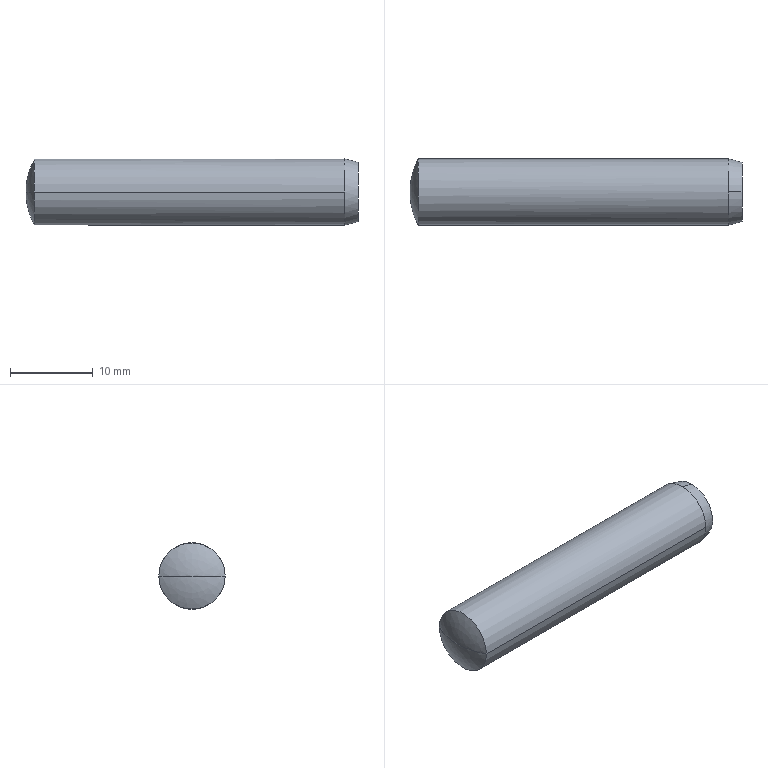Part | STEP file | DIN EN 22338 A - withdrawn 8 m6 x 40 - A | 1 solid | 7 faces | box 40 x 8 x 8 mm | volume 1978 mm3 | spline 2 | cylinder 2 | cone 2 | plane 1 | commonest cylinder face diameters 8 x2
STEP:
#1=CARTESIAN_POINT('',(0.,0.,0.));
#2=DIRECTION('',(0.,0.,1.));
#3=DIRECTION('',(1.,0.,0.));
#4=AXIS2_PLACEMENT_3D('',#1,#2,#3);
#5=CARTESIAN_POINT('',(1.,-4.,0.));
#6=VERTEX_POINT('',#5);
#7=CARTESIAN_POINT('',(1.,4.,0.));
#8=VERTEX_POINT('',#7);
#9=CARTESIAN_POINT('',(1.,0.,0.));
#10=DIRECTION('',(1.,0.,0.));
#11=DIRECTION('',(0.,1.,0.));
#12=AXIS2_PLACEMENT_3D('',#9,#10,#11);
#13=CIRCLE('',#12,4.);
#14=CARTESIAN_POINT('',(1.,-4.,0.));
#15=CARTESIAN_POINT('',(1.,-4.,-8.));
#16=CARTESIAN_POINT('',(1.,4.,-8.));
#17=CARTESIAN_POINT('',(1.,4.,0.));
#18=CARTESIAN_POINT('',(0.3401,-2.763,0.));
#19=CARTESIAN_POINT('',(0.3401,-2.763,-5.525));
#20=CARTESIAN_POINT('',(0.3401,2.763,-5.525));
#21=CARTESIAN_POINT('',(0.3401,2.763,0.));
#22=CARTESIAN_POINT('',(0.,-1.402,0.));
#23=CARTESIAN_POINT('',(0.,-1.402,-2.805));
#24=CARTESIAN_POINT('',(0.,1.402,-2.805));
#25=CARTESIAN_POINT('',(0.,1.402,0.));
#26=CARTESIAN_POINT('',(0.,0.,0.));
#27=CARTESIAN_POINT('',(0.,0.,0.));
#28=CARTESIAN_POINT('',(0.,0.,0.));
#29=CARTESIAN_POINT('',(0.,0.,0.));
#30=(BOUNDED_SURFACE()B_SPLINE_SURFACE(3,3,((#14,#15,#16,#17),(#18,#19,#20,#21),(#22,#23,#24,#25),(#26,#27,#28,#29)),.UNSPECIFIED.,.F.,.F.,.F.)B_SPLINE_SURFACE_WITH_KNOTS((4,4),(4,4),(0.,1.),(0.,1.),.PIECEWISE_BEZIER_KNOTS.)GEOMETRIC_REPRESENTATION_ITEM()RATIONAL_B_SPLINE_SURFACE(((1.,0.3333,0.3333,1.),(0.9801,0.3267,0.3267,0.9801),(0.9801,0.3267,0.3267,0.9801),(1.,0.3333,0.3333,1.)))REPRESENTATION_ITEM('')SURFACE());
#31=CARTESIAN_POINT('',(0.,0.));
#32=CARTESIAN_POINT('',(0.,0.02375));
#33=CARTESIAN_POINT('',(0.,0.06805));
#34=CARTESIAN_POINT('',(0.,0.1267));
#35=CARTESIAN_POINT('',(0.,0.1794));
#36=CARTESIAN_POINT('',(0.,0.2276));
#37=CARTESIAN_POINT('',(0.,0.2721));
#38=CARTESIAN_POINT('',(0.,0.3139));
#39=CARTESIAN_POINT('',(0.,0.3535));
#40=CARTESIAN_POINT('',(0.,0.3914));
#41=CARTESIAN_POINT('',(0.,0.4282));
#42=CARTESIAN_POINT('',(0.,0.4643));
#43=CARTESIAN_POINT('',(0.,0.5));
#44=CARTESIAN_POINT('',(0.,0.5357));
#45=CARTESIAN_POINT('',(0.,0.5718));
#46=CARTESIAN_POINT('',(0.,0.6086));
#47=CARTESIAN_POINT('',(0.,0.6465));
#48=CARTESIAN_POINT('',(0.,0.6861));
#49=CARTESIAN_POINT('',(0.,0.7279));
#50=CARTESIAN_POINT('',(0.,0.7724));
#51=CARTESIAN_POINT('',(0.,0.8206));
#52=CARTESIAN_POINT('',(0.,0.8733));
#53=CARTESIAN_POINT('',(0.,0.9319));
#54=CARTESIAN_POINT('',(0.,0.9763));
#55=CARTESIAN_POINT('',(0.,1.));
#56=B_SPLINE_CURVE_WITH_KNOTS('',3,(#31,#32,#33,#34,#35,#36,#37,#38,#39,#40,#41,#42,#43,#44,#45,#46,#47,#48,#49,#50,#51,#52,#53,#54,#55),.UNSPECIFIED.,.F.,.F.,(4,1,1,1,1,1,1,1,1,1,1,1,1,1,1,1,1,1,1,1,1,1,4),(3.142,3.284,3.427,3.57,3.713,3.856,3.998,4.141,4.284,4.427,4.57,4.712,4.855,4.998,5.141,5.284,5.426,5.569,5.712,5.855,5.998,6.14,6.283),.QUASI_UNIFORM_KNOTS.);
#57=(GEOMETRIC_REPRESENTATION_CONTEXT(2)PARAMETRIC_REPRESENTATION_CONTEXT()REPRESENTATION_CONTEXT('',''));
#58=DEFINITIONAL_REPRESENTATION('',(#56),#57);
#59=PCURVE('',#30,#58);
#60=CARTESIAN_POINT('',(19.7,0.,0.));
#61=DIRECTION('',(1.,0.,0.));
#62=DIRECTION('',(0.,1.,0.));
#63=AXIS2_PLACEMENT_3D('',#60,#61,#62);
#64=CYLINDRICAL_SURFACE('',#63,4.);
#65=CARTESIAN_POINT('',(0.,-18.7));
#66=DIRECTION('',(1.,0.));
#67=VECTOR('',#66,1.);
#68=LINE('',#65,#67);
#69=(GEOMETRIC_REPRESENTATION_CONTEXT(2)PARAMETRIC_REPRESENTATION_CONTEXT()REPRESENTATION_CONTEXT('',''));
#70=DEFINITIONAL_REPRESENTATION('',(#68),#69);
#71=PCURVE('',#64,#70);
#72=SURFACE_CURVE('',#13,(#59,#71),.PCURVE_S1.);
#73=EDGE_CURVE('',#6,#8,#72,.T.);
#74=ORIENTED_EDGE('',*,*,#73,.F.);
#75=CARTESIAN_POINT('',(0.,0.,0.));
#76=VERTEX_POINT('',#75);
#77=CARTESIAN_POINT('',(8.5,0.,0.));
#78=DIRECTION('',(0.,0.,-1.));
#79=DIRECTION('',(1.,0.,0.));
#80=AXIS2_PLACEMENT_3D('',#77,#78,#79);
#81=CIRCLE('',#80,8.5);
#82=CARTESIAN_POINT('',(0.,0.));
#83=CARTESIAN_POINT('',(0.0153,0.));
#84=CARTESIAN_POINT('',(0.04587,0.));
#85=CARTESIAN_POINT('',(0.09161,0.));
#86=CARTESIAN_POINT('',(0.1372,0.));
#87=CARTESIAN_POINT('',(0.1828,0.));
#88=CARTESIAN_POINT('',(0.2282,0.));
#89=CARTESIAN_POINT('',(0.2736,0.));
#90=CARTESIAN_POINT('',(0.319,0.));
#91=CARTESIAN_POINT('',(0.3643,0.));
#92=CARTESIAN_POINT('',(0.4095,0.));
#93=CARTESIAN_POINT('',(0.4548,0.));
#94=CARTESIAN_POINT('',(0.5,0.));
#95=CARTESIAN_POINT('',(0.5452,0.));
#96=CARTESIAN_POINT('',(0.5905,0.));
#97=CARTESIAN_POINT('',(0.6357,0.));
#98=CARTESIAN_POINT('',(0.681,0.));
#99=CARTESIAN_POINT('',(0.7264,0.));
#100=CARTESIAN_POINT('',(0.7718,0.));
#101=CARTESIAN_POINT('',(0.8172,0.));
#102=CARTESIAN_POINT('',(0.8628,0.));
#103=CARTESIAN_POINT('',(0.9084,0.));
#104=CARTESIAN_POINT('',(0.9541,0.));
#105=CARTESIAN_POINT('',(0.9847,0.));
#106=CARTESIAN_POINT('',(1.,0.));
#107=B_SPLINE_CURVE_WITH_KNOTS('',3,(#82,#83,#84,#85,#86,#87,#88,#89,#90,#91,#92,#93,#94,#95,#96,#97,#98,#99,#100,#101,#102,#103,#104,#105,#106),.UNSPECIFIED.,.F.,.F.,(4,1,1,1,1,1,1,1,1,1,1,1,1,1,1,1,1,1,1,1,1,1,4),(2.652,2.674,2.696,2.718,2.741,2.763,2.785,2.808,2.83,2.852,2.874,2.897,2.919,2.941,2.963,2.986,3.008,3.03,3.053,3.075,3.097,3.119,3.142),.QUASI_UNIFORM_KNOTS.);
#108=(GEOMETRIC_REPRESENTATION_CONTEXT(2)PARAMETRIC_REPRESENTATION_CONTEXT()REPRESENTATION_CONTEXT('',''));
#109=DEFINITIONAL_REPRESENTATION('',(#107),#108);
#110=PCURVE('',#30,#109);
#111=CARTESIAN_POINT('',(1.,4.,0.));
#112=CARTESIAN_POINT('',(1.,4.,8.));
#113=CARTESIAN_POINT('',(1.,-4.,8.));
#114=CARTESIAN_POINT('',(1.,-4.,0.));
#115=CARTESIAN_POINT('',(0.3401,2.763,0.));
#116=CARTESIAN_POINT('',(0.3401,2.763,5.525));
#117=CARTESIAN_POINT('',(0.3401,-2.763,5.525));
#118=CARTESIAN_POINT('',(0.3401,-2.763,0.));
#119=CARTESIAN_POINT('',(0.,1.402,0.));
#120=CARTESIAN_POINT('',(0.,1.402,2.805));
#121=CARTESIAN_POINT('',(0.,-1.402,2.805));
#122=CARTESIAN_POINT('',(0.,-1.402,0.));
#123=CARTESIAN_POINT('',(0.,0.,0.));
#124=CARTESIAN_POINT('',(0.,0.,0.));
#125=CARTESIAN_POINT('',(0.,0.,0.));
#126=CARTESIAN_POINT('',(0.,0.,0.));
#127=(BOUNDED_SURFACE()B_SPLINE_SURFACE(3,3,((#111,#112,#113,#114),(#115,#116,#117,#118),(#119,#120,#121,#122),(#123,#124,#125,#126)),.UNSPECIFIED.,.F.,.F.,.F.)B_SPLINE_SURFACE_WITH_KNOTS((4,4),(4,4),(0.,1.),(0.,1.),.PIECEWISE_BEZIER_KNOTS.)GEOMETRIC_REPRESENTATION_ITEM()RATIONAL_B_SPLINE_SURFACE(((1.,0.3333,0.3333,1.),(0.9801,0.3267,0.3267,0.9801),(0.9801,0.3267,0.3267,0.9801),(1.,0.3333,0.3333,1.)))REPRESENTATION_ITEM('')SURFACE());
#128=CARTESIAN_POINT('',(0.,1.));
#129=CARTESIAN_POINT('',(0.0153,1.));
#130=CARTESIAN_POINT('',(0.04587,1.));
#131=CARTESIAN_POINT('',(0.09161,1.));
#132=CARTESIAN_POINT('',(0.1372,1.));
#133=CARTESIAN_POINT('',(0.1828,1.));
#134=CARTESIAN_POINT('',(0.2282,1.));
#135=CARTESIAN_POINT('',(0.2736,1.));
#136=CARTESIAN_POINT('',(0.319,1.));
#137=CARTESIAN_POINT('',(0.3643,1.));
#138=CARTESIAN_POINT('',(0.4095,1.));
#139=CARTESIAN_POINT('',(0.4548,1.));
#140=CARTESIAN_POINT('',(0.5,1.));
#141=CARTESIAN_POINT('',(0.5452,1.));
#142=CARTESIAN_POINT('',(0.5905,1.));
#143=CARTESIAN_POINT('',(0.6357,1.));
#144=CARTESIAN_POINT('',(0.681,1.));
#145=CARTESIAN_POINT('',(0.7264,1.));
#146=CARTESIAN_POINT('',(0.7718,1.));
#147=CARTESIAN_POINT('',(0.8172,1.));
#148=CARTESIAN_POINT('',(0.8628,1.));
#149=CARTESIAN_POINT('',(0.9084,1.));
#150=CARTESIAN_POINT('',(0.9541,1.));
#151=CARTESIAN_POINT('',(0.9847,1.));
#152=CARTESIAN_POINT('',(1.,1.));
#153=B_SPLINE_CURVE_WITH_KNOTS('',3,(#128,#129,#130,#131,#132,#133,#134,#135,#136,#137,#138,#139,#140,#141,#142,#143,#144,#145,#146,#147,#148,#149,#150,#151,#152),.UNSPECIFIED.,.F.,.F.,(4,1,1,1,1,1,1,1,1,1,1,1,1,1,1,1,1,1,1,1,1,1,4),(2.652,2.674,2.696,2.718,2.741,2.763,2.785,2.808,2.83,2.852,2.874,2.897,2.919,2.941,2.963,2.986,3.008,3.03,3.053,3.075,3.097,3.119,3.142),.QUASI_UNIFORM_KNOTS.);
#154=(GEOMETRIC_REPRESENTATION_CONTEXT(2)PARAMETRIC_REPRESENTATION_CONTEXT()REPRESENTATION_CONTEXT('',''));
#155=DEFINITIONAL_REPRESENTATION('',(#153),#154);
#156=PCURVE('',#127,#155);
#157=SURFACE_CURVE('',#81,(#110,#156),.PCURVE_S1.);
#158=EDGE_CURVE('',#6,#76,#157,.T.);
#159=ORIENTED_EDGE('',*,*,#158,.T.);
#160=CARTESIAN_POINT('',(8.5,0.,0.));
#161=DIRECTION('',(0.,0.,1.));
#162=DIRECTION('',(1.,0.,0.));
#163=AXIS2_PLACEMENT_3D('',#160,#161,#162);
#164=CIRCLE('',#163,8.5);
#165=CARTESIAN_POINT('',(0.,1.));
#166=CARTESIAN_POINT('',(0.0153,1.));
#167=CARTESIAN_POINT('',(0.04587,1.));
#168=CARTESIAN_POINT('',(0.09161,1.));
#169=CARTESIAN_POINT('',(0.1372,1.));
#170=CARTESIAN_POINT('',(0.1828,1.));
#171=CARTESIAN_POINT('',(0.2282,1.));
#172=CARTESIAN_POINT('',(0.2736,1.));
#173=CARTESIAN_POINT('',(0.319,1.));
#174=CARTESIAN_POINT('',(0.3643,1.));
#175=CARTESIAN_POINT('',(0.4095,1.));
#176=CARTESIAN_POINT('',(0.4548,1.));
#177=CARTESIAN_POINT('',(0.5,1.));
#178=CARTESIAN_POINT('',(0.5452,1.));
#179=CARTESIAN_POINT('',(0.5905,1.));
#180=CARTESIAN_POINT('',(0.6357,1.));
#181=CARTESIAN_POINT('',(0.681,1.));
#182=CARTESIAN_POINT('',(0.7264,1.));
#183=CARTESIAN_POINT('',(0.7718,1.));
#184=CARTESIAN_POINT('',(0.8172,1.));
#185=CARTESIAN_POINT('',(0.8628,1.));
#186=CARTESIAN_POINT('',(0.9084,1.));
#187=CARTESIAN_POINT('',(0.9541,1.));
#188=CARTESIAN_POINT('',(0.9847,1.));
#189=CARTESIAN_POINT('',(1.,1.));
#190=B_SPLINE_CURVE_WITH_KNOTS('',3,(#165,#166,#167,#168,#169,#170,#171,#172,#173,#174,#175,#176,#177,#178,#179,#180,#181,#182,#183,#184,#185,#186,#187,#188,#189),.UNSPECIFIED.,.F.,.F.,(4,1,1,1,1,1,1,1,1,1,1,1,1,1,1,1,1,1,1,1,1,1,4),(2.652,2.674,2.696,2.718,2.741,2.763,2.785,2.808,2.83,2.852,2.874,2.897,2.919,2.941,2.963,2.986,3.008,3.03,3.053,3.075,3.097,3.119,3.142),.QUASI_UNIFORM_KNOTS.);
#191=(GEOMETRIC_REPRESENTATION_CONTEXT(2)PARAMETRIC_REPRESENTATION_CONTEXT()REPRESENTATION_CONTEXT('',''));
#192=DEFINITIONAL_REPRESENTATION('',(#190),#191);
#193=PCURVE('',#30,#192);
#194=CARTESIAN_POINT('',(0.,0.));
#195=CARTESIAN_POINT('',(0.0153,0.));
#196=CARTESIAN_POINT('',(0.04587,0.));
#197=CARTESIAN_POINT('',(0.09161,0.));
#198=CARTESIAN_POINT('',(0.1372,0.));
#199=CARTESIAN_POINT('',(0.1828,0.));
#200=CARTESIAN_POINT('',(0.2282,0.));
#201=CARTESIAN_POINT('',(0.2736,0.));
#202=CARTESIAN_POINT('',(0.319,0.));
#203=CARTESIAN_POINT('',(0.3643,0.));
#204=CARTESIAN_POINT('',(0.4095,0.));
#205=CARTESIAN_POINT('',(0.4548,0.));
#206=CARTESIAN_POINT('',(0.5,0.));
#207=CARTESIAN_POINT('',(0.5452,0.));
#208=CARTESIAN_POINT('',(0.5905,0.));
#209=CARTESIAN_POINT('',(0.6357,0.));
#210=CARTESIAN_POINT('',(0.681,0.));
#211=CARTESIAN_POINT('',(0.7264,0.));
#212=CARTESIAN_POINT('',(0.7718,0.));
#213=CARTESIAN_POINT('',(0.8172,0.));
#214=CARTESIAN_POINT('',(0.8628,0.));
#215=CARTESIAN_POINT('',(0.9084,0.));
#216=CARTESIAN_POINT('',(0.9541,0.));
#217=CARTESIAN_POINT('',(0.9847,0.));
#218=CARTESIAN_POINT('',(1.,0.));
#219=B_SPLINE_CURVE_WITH_KNOTS('',3,(#194,#195,#196,#197,#198,#199,#200,#201,#202,#203,#204,#205,#206,#207,#208,#209,#210,#211,#212,#213,#214,#215,#216,#217,#218),.UNSPECIFIED.,.F.,.F.,(4,1,1,1,1,1,1,1,1,1,1,1,1,1,1,1,1,1,1,1,1,1,4),(2.652,2.674,2.696,2.718,2.741,2.763,2.785,2.808,2.83,2.852,2.874,2.897,2.919,2.941,2.963,2.986,3.008,3.03,3.053,3.075,3.097,3.119,3.142),.QUASI_UNIFORM_KNOTS.);
#220=(GEOMETRIC_REPRESENTATION_CONTEXT(2)PARAMETRIC_REPRESENTATION_CONTEXT()REPRESENTATION_CONTEXT('',''));
#221=DEFINITIONAL_REPRESENTATION('',(#219),#220);
#222=PCURVE('',#127,#221);
#223=SURFACE_CURVE('',#164,(#193,#222),.PCURVE_S1.);
#224=EDGE_CURVE('',#8,#76,#223,.T.);
#225=ORIENTED_EDGE('',*,*,#224,.F.);
#226=EDGE_LOOP('',(#74,#159,#225));
#227=FACE_BOUND('',#226,.T.);
#228=ADVANCED_FACE('',(#227),#30,.T.);
#229=CARTESIAN_POINT('',(1.,0.,0.));
#230=DIRECTION('',(1.,0.,0.));
#231=DIRECTION('',(0.,1.,0.));
#232=AXIS2_PLACEMENT_3D('',#229,#230,#231);
#233=CIRCLE('',#232,4.);
#234=CARTESIAN_POINT('',(19.7,0.,0.));
#235=DIRECTION('',(1.,0.,0.));
#236=DIRECTION('',(0.,1.,0.));
#237=AXIS2_PLACEMENT_3D('',#234,#235,#236);
#238=CYLINDRICAL_SURFACE('',#237,4.);
#239=CARTESIAN_POINT('',(0.,-18.7));
#240=DIRECTION('',(1.,0.));
#241=VECTOR('',#240,1.);
#242=LINE('',#239,#241);
#243=(GEOMETRIC_REPRESENTATION_CONTEXT(2)PARAMETRIC_REPRESENTATION_CONTEXT()REPRESENTATION_CONTEXT('',''));
#244=DEFINITIONAL_REPRESENTATION('',(#242),#243);
#245=PCURVE('',#238,#244);
#246=CARTESIAN_POINT('',(0.,0.));
#247=CARTESIAN_POINT('',(0.,0.02375));
#248=CARTESIAN_POINT('',(0.,0.06805));
#249=CARTESIAN_POINT('',(0.,0.1267));
#250=CARTESIAN_POINT('',(0.,0.1794));
#251=CARTESIAN_POINT('',(0.,0.2276));
#252=CARTESIAN_POINT('',(0.,0.2721));
#253=CARTESIAN_POINT('',(0.,0.3139));
#254=CARTESIAN_POINT('',(0.,0.3535));
#255=CARTESIAN_POINT('',(0.,0.3914));
#256=CARTESIAN_POINT('',(0.,0.4282));
#257=CARTESIAN_POINT('',(0.,0.4643));
#258=CARTESIAN_POINT('',(0.,0.5));
#259=CARTESIAN_POINT('',(0.,0.5357));
#260=CARTESIAN_POINT('',(0.,0.5718));
#261=CARTESIAN_POINT('',(0.,0.6086));
#262=CARTESIAN_POINT('',(0.,0.6465));
#263=CARTESIAN_POINT('',(0.,0.6861));
#264=CARTESIAN_POINT('',(0.,0.7279));
#265=CARTESIAN_POINT('',(0.,0.7724));
#266=CARTESIAN_POINT('',(0.,0.8206));
#267=CARTESIAN_POINT('',(0.,0.8733));
#268=CARTESIAN_POINT('',(0.,0.9319));
#269=CARTESIAN_POINT('',(0.,0.9763));
#270=CARTESIAN_POINT('',(0.,1.));
#271=B_SPLINE_CURVE_WITH_KNOTS('',3,(#246,#247,#248,#249,#250,#251,#252,#253,#254,#255,#256,#257,#258,#259,#260,#261,#262,#263,#264,#265,#266,#267,#268,#269,#270),.UNSPECIFIED.,.F.,.F.,(4,1,1,1,1,1,1,1,1,1,1,1,1,1,1,1,1,1,1,1,1,1,4),(0.,0.1428,0.2856,0.4284,0.5712,0.714,0.8568,0.9996,1.142,1.285,1.428,1.571,1.714,1.856,1.999,2.142,2.285,2.428,2.57,2.713,2.856,2.999,3.142),.QUASI_UNIFORM_KNOTS.);
#272=(GEOMETRIC_REPRESENTATION_CONTEXT(2)PARAMETRIC_REPRESENTATION_CONTEXT()REPRESENTATION_CONTEXT('',''));
#273=DEFINITIONAL_REPRESENTATION('',(#271),#272);
#274=PCURVE('',#127,#273);
#275=SURFACE_CURVE('',#233,(#245,#274),.PCURVE_S1.);
#276=EDGE_CURVE('',#8,#6,#275,.T.);
#277=ORIENTED_EDGE('',*,*,#276,.T.);
#278=CARTESIAN_POINT('',(38.4,-4.,0.));
#279=VERTEX_POINT('',#278);
#280=CARTESIAN_POINT('',(19.7,-4.,0.));
#281=DIRECTION('',(1.,0.,0.));
#282=VECTOR('',#281,1.);
#283=LINE('',#280,#282);
#284=CARTESIAN_POINT('',(3.142,0.));
#285=DIRECTION('',(0.,1.));
#286=VECTOR('',#285,1.);
#287=LINE('',#284,#286);
#288=(GEOMETRIC_REPRESENTATION_CONTEXT(2)PARAMETRIC_REPRESENTATION_CONTEXT()REPRESENTATION_CONTEXT('',''));
#289=DEFINITIONAL_REPRESENTATION('',(#287),#288);
#290=PCURVE('',#238,#289);
#291=CARTESIAN_POINT('',(3.142,0.));
#292=DIRECTION('',(0.,1.));
#293=VECTOR('',#292,1.);
#294=LINE('',#291,#293);
#295=(GEOMETRIC_REPRESENTATION_CONTEXT(2)PARAMETRIC_REPRESENTATION_CONTEXT()REPRESENTATION_CONTEXT('',''));
#296=DEFINITIONAL_REPRESENTATION('',(#294),#295);
#297=PCURVE('',#64,#296);
#298=SURFACE_CURVE('',#283,(#290,#297),.PCURVE_S1.);
#299=EDGE_CURVE('',#6,#279,#298,.T.);
#300=ORIENTED_EDGE('',*,*,#299,.T.);
#301=CARTESIAN_POINT('',(38.4,0.,4.));
#302=VERTEX_POINT('',#301);
#303=CARTESIAN_POINT('',(38.4,0.,0.));
#304=DIRECTION('',(-1.,0.,0.));
#305=DIRECTION('',(0.,1.,0.));
#306=AXIS2_PLACEMENT_3D('',#303,#304,#305);
#307=CIRCLE('',#306,4.);
#308=CARTESIAN_POINT('',(6.283,18.7));
#309=DIRECTION('',(-1.,0.));
#310=VECTOR('',#309,1.);
#311=LINE('',#308,#310);
#312=(GEOMETRIC_REPRESENTATION_CONTEXT(2)PARAMETRIC_REPRESENTATION_CONTEXT()REPRESENTATION_CONTEXT('',''));
#313=DEFINITIONAL_REPRESENTATION('',(#311),#312);
#314=PCURVE('',#238,#313);
#315=CARTESIAN_POINT('',(38.4,0.,0.));
#316=DIRECTION('',(-1.,0.,0.));
#317=DIRECTION('',(0.,0.,1.));
#318=AXIS2_PLACEMENT_3D('',#315,#316,#317);
#319=CONICAL_SURFACE('',#318,4.,0.2618);
#320=CARTESIAN_POINT('',(1.571,0.));
#321=DIRECTION('',(1.,0.));
#322=VECTOR('',#321,1.);
#323=LINE('',#320,#322);
#324=(GEOMETRIC_REPRESENTATION_CONTEXT(2)PARAMETRIC_REPRESENTATION_CONTEXT()REPRESENTATION_CONTEXT('',''));
#325=DEFINITIONAL_REPRESENTATION('',(#323),#324);
#326=PCURVE('',#319,#325);
#327=SURFACE_CURVE('',#307,(#314,#326),.PCURVE_S1.);
#328=EDGE_CURVE('',#279,#302,#327,.T.);
#329=ORIENTED_EDGE('',*,*,#328,.T.);
#330=CARTESIAN_POINT('',(38.4,4.,0.));
#331=VERTEX_POINT('',#330);
#332=CARTESIAN_POINT('',(38.4,0.,0.));
#333=DIRECTION('',(-1.,0.,0.));
#334=DIRECTION('',(0.,1.,0.));
#335=AXIS2_PLACEMENT_3D('',#332,#333,#334);
#336=CIRCLE('',#335,4.);
#337=CARTESIAN_POINT('',(6.283,18.7));
#338=DIRECTION('',(-1.,0.));
#339=VECTOR('',#338,1.);
#340=LINE('',#337,#339);
#341=(GEOMETRIC_REPRESENTATION_CONTEXT(2)PARAMETRIC_REPRESENTATION_CONTEXT()REPRESENTATION_CONTEXT('',''));
#342=DEFINITIONAL_REPRESENTATION('',(#340),#341);
#343=PCURVE('',#238,#342);
#344=CARTESIAN_POINT('',(38.4,0.,0.));
#345=DIRECTION('',(-1.,0.,0.));
#346=DIRECTION('',(0.,0.,1.));
#347=AXIS2_PLACEMENT_3D('',#344,#345,#346);
#348=CONICAL_SURFACE('',#347,4.,0.2618);
#349=CARTESIAN_POINT('',(-4.712,0.));
#350=DIRECTION('',(1.,0.));
#351=VECTOR('',#350,1.);
#352=LINE('',#349,#351);
#353=(GEOMETRIC_REPRESENTATION_CONTEXT(2)PARAMETRIC_REPRESENTATION_CONTEXT()REPRESENTATION_CONTEXT('',''));
#354=DEFINITIONAL_REPRESENTATION('',(#352),#353);
#355=PCURVE('',#348,#354);
#356=SURFACE_CURVE('',#336,(#343,#355),.PCURVE_S1.);
#357=EDGE_CURVE('',#302,#331,#356,.T.);
#358=ORIENTED_EDGE('',*,*,#357,.T.);
#359=CARTESIAN_POINT('',(19.7,4.,0.));
#360=DIRECTION('',(1.,0.,0.));
#361=VECTOR('',#360,1.);
#362=LINE('',#359,#361);
#363=CARTESIAN_POINT('',(0.,0.));
#364=DIRECTION('',(0.,1.));
#365=VECTOR('',#364,1.);
#366=LINE('',#363,#365);
#367=(GEOMETRIC_REPRESENTATION_CONTEXT(2)PARAMETRIC_REPRESENTATION_CONTEXT()REPRESENTATION_CONTEXT('',''));
#368=DEFINITIONAL_REPRESENTATION('',(#366),#367);
#369=PCURVE('',#238,#368);
#370=CARTESIAN_POINT('',(6.283,0.));
#371=DIRECTION('',(0.,1.));
#372=VECTOR('',#371,1.);
#373=LINE('',#370,#372);
#374=(GEOMETRIC_REPRESENTATION_CONTEXT(2)PARAMETRIC_REPRESENTATION_CONTEXT()REPRESENTATION_CONTEXT('',''));
#375=DEFINITIONAL_REPRESENTATION('',(#373),#374);
#376=PCURVE('',#64,#375);
#377=SURFACE_CURVE('',#362,(#369,#376),.PCURVE_S1.);
#378=EDGE_CURVE('',#8,#331,#377,.T.);
#379=ORIENTED_EDGE('',*,*,#378,.F.);
#380=EDGE_LOOP('',(#277,#300,#329,#358,#379));
#381=FACE_BOUND('',#380,.T.);
#382=ADVANCED_FACE('',(#381),#238,.T.);
#383=CARTESIAN_POINT('',(40.,0.,3.571));
#384=VERTEX_POINT('',#383);
#385=CARTESIAN_POINT('',(40.,0.,-3.571));
#386=VERTEX_POINT('',#385);
#387=CARTESIAN_POINT('',(40.,0.,0.));
#388=DIRECTION('',(-1.,0.,0.));
#389=DIRECTION('',(0.,0.,1.));
#390=AXIS2_PLACEMENT_3D('',#387,#388,#389);
#391=CIRCLE('',#390,3.571);
#392=CARTESIAN_POINT('',(0.,-1.6));
#393=DIRECTION('',(1.,0.));
#394=VECTOR('',#393,1.);
#395=LINE('',#392,#394);
#396=(GEOMETRIC_REPRESENTATION_CONTEXT(2)PARAMETRIC_REPRESENTATION_CONTEXT()REPRESENTATION_CONTEXT('',''));
#397=DEFINITIONAL_REPRESENTATION('',(#395),#396);
#398=PCURVE('',#348,#397);
#399=CARTESIAN_POINT('',(40.,1.786,0.));
#400=DIRECTION('',(1.,0.,0.));
#401=DIRECTION('',(0.,0.,-1.));
#402=AXIS2_PLACEMENT_3D('',#399,#400,#401);
#403=PLANE('',#402);
#404=CARTESIAN_POINT('',(-3.571,-1.786));
#405=CARTESIAN_POINT('',(-3.571,4.4));
#406=CARTESIAN_POINT('',(1.786,1.307));
#407=CARTESIAN_POINT('',(7.143,-1.786));
#408=CARTESIAN_POINT('',(1.786,-4.878));
#409=CARTESIAN_POINT('',(-3.571,-7.971));
#410=CARTESIAN_POINT('',(-3.571,-1.786));
#411=(BOUNDED_CURVE()B_SPLINE_CURVE(2,(#404,#405,#406,#407,#408,#409,#410),.UNSPECIFIED.,.T.,.F.)B_SPLINE_CURVE_WITH_KNOTS((1,2,2,2,2,1),(-2.094,0.,2.094,4.189,6.283,8.378),.UNSPECIFIED.)CURVE()GEOMETRIC_REPRESENTATION_ITEM()RATIONAL_B_SPLINE_CURVE((1.,0.5,1.,0.5,1.,0.5,1.))REPRESENTATION_ITEM(''));
#412=(GEOMETRIC_REPRESENTATION_CONTEXT(2)PARAMETRIC_REPRESENTATION_CONTEXT()REPRESENTATION_CONTEXT('',''));
#413=DEFINITIONAL_REPRESENTATION('',(#411),#412);
#414=PCURVE('',#403,#413);
#415=SURFACE_CURVE('',#391,(#398,#414),.PCURVE_S1.);
#416=EDGE_CURVE('',#384,#386,#415,.T.);
#417=ORIENTED_EDGE('',*,*,#416,.T.);
#418=CARTESIAN_POINT('',(38.4,0.,-4.));
#419=VERTEX_POINT('',#418);
#420=CARTESIAN_POINT('',(38.4,0.,-4.));
#421=DIRECTION('',(-0.9659,0.,-0.2588));
#422=VECTOR('',#421,1.);
#423=LINE('',#420,#422);
#424=CARTESIAN_POINT('',(3.142,0.));
#425=DIRECTION('',(0.,1.));
#426=VECTOR('',#425,1.);
#427=LINE('',#424,#426);
#428=(GEOMETRIC_REPRESENTATION_CONTEXT(2)PARAMETRIC_REPRESENTATION_CONTEXT()REPRESENTATION_CONTEXT('',''));
#429=DEFINITIONAL_REPRESENTATION('',(#427),#428);
#430=PCURVE('',#348,#429);
#431=CARTESIAN_POINT('',(3.142,0.));
#432=DIRECTION('',(0.,1.));
#433=VECTOR('',#432,1.);
#434=LINE('',#431,#433);
#435=(GEOMETRIC_REPRESENTATION_CONTEXT(2)PARAMETRIC_REPRESENTATION_CONTEXT()REPRESENTATION_CONTEXT('',''));
#436=DEFINITIONAL_REPRESENTATION('',(#434),#435);
#437=PCURVE('',#319,#436);
#438=SURFACE_CURVE('',#423,(#430,#437),.PCURVE_S1.);
#439=EDGE_CURVE('',#386,#419,#438,.T.);
#440=ORIENTED_EDGE('',*,*,#439,.T.);
#441=CARTESIAN_POINT('',(38.4,0.,0.));
#442=DIRECTION('',(-1.,0.,0.));
#443=DIRECTION('',(0.,1.,0.));
#444=AXIS2_PLACEMENT_3D('',#441,#442,#443);
#445=CIRCLE('',#444,4.);
#446=CARTESIAN_POINT('',(1.571,0.));
#447=DIRECTION('',(1.,0.));
#448=VECTOR('',#447,1.);
#449=LINE('',#446,#448);
#450=(GEOMETRIC_REPRESENTATION_CONTEXT(2)PARAMETRIC_REPRESENTATION_CONTEXT()REPRESENTATION_CONTEXT('',''));
#451=DEFINITIONAL_REPRESENTATION('',(#449),#450);
#452=PCURVE('',#348,#451);
#453=CARTESIAN_POINT('',(6.283,18.7));
#454=DIRECTION('',(-1.,0.));
#455=VECTOR('',#454,1.);
#456=LINE('',#453,#455);
#457=(GEOMETRIC_REPRESENTATION_CONTEXT(2)PARAMETRIC_REPRESENTATION_CONTEXT()REPRESENTATION_CONTEXT('',''));
#458=DEFINITIONAL_REPRESENTATION('',(#456),#457);
#459=PCURVE('',#64,#458);
#460=SURFACE_CURVE('',#445,(#452,#459),.PCURVE_S1.);
#461=EDGE_CURVE('',#331,#419,#460,.T.);
#462=ORIENTED_EDGE('',*,*,#461,.F.);
#463=ORIENTED_EDGE('',*,*,#357,.F.);
#464=CARTESIAN_POINT('',(38.4,0.,4.));
#465=DIRECTION('',(-0.9659,0.,0.2588));
#466=VECTOR('',#465,1.);
#467=LINE('',#464,#466);
#468=CARTESIAN_POINT('',(0.,0.));
#469=DIRECTION('',(0.,1.));
#470=VECTOR('',#469,1.);
#471=LINE('',#468,#470);
#472=(GEOMETRIC_REPRESENTATION_CONTEXT(2)PARAMETRIC_REPRESENTATION_CONTEXT()REPRESENTATION_CONTEXT('',''));
#473=DEFINITIONAL_REPRESENTATION('',(#471),#472);
#474=PCURVE('',#348,#473);
#475=CARTESIAN_POINT('',(6.283,0.));
#476=DIRECTION('',(0.,1.));
#477=VECTOR('',#476,1.);
#478=LINE('',#475,#477);
#479=(GEOMETRIC_REPRESENTATION_CONTEXT(2)PARAMETRIC_REPRESENTATION_CONTEXT()REPRESENTATION_CONTEXT('',''));
#480=DEFINITIONAL_REPRESENTATION('',(#478),#479);
#481=PCURVE('',#319,#480);
#482=SURFACE_CURVE('',#467,(#474,#481),.PCURVE_S1.);
#483=EDGE_CURVE('',#384,#302,#482,.T.);
#484=ORIENTED_EDGE('',*,*,#483,.F.);
#485=EDGE_LOOP('',(#417,#440,#462,#463,#484));
#486=FACE_BOUND('',#485,.T.);
#487=ADVANCED_FACE('',(#486),#348,.T.);
#488=ORIENTED_EDGE('',*,*,#299,.F.);
#489=ORIENTED_EDGE('',*,*,#73,.T.);
#490=ORIENTED_EDGE('',*,*,#378,.T.);
#491=ORIENTED_EDGE('',*,*,#461,.T.);
#492=CARTESIAN_POINT('',(38.4,0.,0.));
#493=DIRECTION('',(-1.,0.,0.));
#494=DIRECTION('',(0.,1.,0.));
#495=AXIS2_PLACEMENT_3D('',#492,#493,#494);
#496=CIRCLE('',#495,4.);
#497=CARTESIAN_POINT('',(6.283,18.7));
#498=DIRECTION('',(-1.,0.));
#499=VECTOR('',#498,1.);
#500=LINE('',#497,#499);
#501=(GEOMETRIC_REPRESENTATION_CONTEXT(2)PARAMETRIC_REPRESENTATION_CONTEXT()REPRESENTATION_CONTEXT('',''));
#502=DEFINITIONAL_REPRESENTATION('',(#500),#501);
#503=PCURVE('',#64,#502);
#504=CARTESIAN_POINT('',(1.571,0.));
#505=DIRECTION('',(1.,0.));
#506=VECTOR('',#505,1.);
#507=LINE('',#504,#506);
#508=(GEOMETRIC_REPRESENTATION_CONTEXT(2)PARAMETRIC_REPRESENTATION_CONTEXT()REPRESENTATION_CONTEXT('',''));
#509=DEFINITIONAL_REPRESENTATION('',(#507),#508);
#510=PCURVE('',#319,#509);
#511=SURFACE_CURVE('',#496,(#503,#510),.PCURVE_S1.);
#512=EDGE_CURVE('',#419,#279,#511,.T.);
#513=ORIENTED_EDGE('',*,*,#512,.T.);
#514=EDGE_LOOP('',(#488,#489,#490,#491,#513));
#515=FACE_BOUND('',#514,.T.);
#516=ADVANCED_FACE('',(#515),#64,.T.);
#517=ORIENTED_EDGE('',*,*,#158,.F.);
#518=ORIENTED_EDGE('',*,*,#276,.F.);
#519=ORIENTED_EDGE('',*,*,#224,.T.);
#520=EDGE_LOOP('',(#517,#518,#519));
#521=FACE_BOUND('',#520,.T.);
#522=ADVANCED_FACE('',(#521),#127,.T.);
#523=ORIENTED_EDGE('',*,*,#439,.F.);
#524=CARTESIAN_POINT('',(40.,0.,0.));
#525=DIRECTION('',(-1.,0.,0.));
#526=DIRECTION('',(0.,0.,1.));
#527=AXIS2_PLACEMENT_3D('',#524,#525,#526);
#528=CIRCLE('',#527,3.571);
#529=CARTESIAN_POINT('',(0.,-1.6));
#530=DIRECTION('',(1.,0.));
#531=VECTOR('',#530,1.);
#532=LINE('',#529,#531);
#533=(GEOMETRIC_REPRESENTATION_CONTEXT(2)PARAMETRIC_REPRESENTATION_CONTEXT()REPRESENTATION_CONTEXT('',''));
#534=DEFINITIONAL_REPRESENTATION('',(#532),#533);
#535=PCURVE('',#319,#534);
#536=CARTESIAN_POINT('',(-3.571,-1.786));
#537=CARTESIAN_POINT('',(-3.571,4.4));
#538=CARTESIAN_POINT('',(1.786,1.307));
#539=CARTESIAN_POINT('',(7.143,-1.786));
#540=CARTESIAN_POINT('',(1.786,-4.878));
#541=CARTESIAN_POINT('',(-3.571,-7.971));
#542=CARTESIAN_POINT('',(-3.571,-1.786));
#543=(BOUNDED_CURVE()B_SPLINE_CURVE(2,(#536,#537,#538,#539,#540,#541,#542),.UNSPECIFIED.,.T.,.F.)B_SPLINE_CURVE_WITH_KNOTS((1,2,2,2,2,1),(-2.094,0.,2.094,4.189,6.283,8.378),.UNSPECIFIED.)CURVE()GEOMETRIC_REPRESENTATION_ITEM()RATIONAL_B_SPLINE_CURVE((1.,0.5,1.,0.5,1.,0.5,1.))REPRESENTATION_ITEM(''));
#544=(GEOMETRIC_REPRESENTATION_CONTEXT(2)PARAMETRIC_REPRESENTATION_CONTEXT()REPRESENTATION_CONTEXT('',''));
#545=DEFINITIONAL_REPRESENTATION('',(#543),#544);
#546=PCURVE('',#403,#545);
#547=SURFACE_CURVE('',#528,(#535,#546),.PCURVE_S1.);
#548=EDGE_CURVE('',#386,#384,#547,.T.);
#549=ORIENTED_EDGE('',*,*,#548,.T.);
#550=ORIENTED_EDGE('',*,*,#483,.T.);
#551=ORIENTED_EDGE('',*,*,#328,.F.);
#552=ORIENTED_EDGE('',*,*,#512,.F.);
#553=EDGE_LOOP('',(#523,#549,#550,#551,#552));
#554=FACE_BOUND('',#553,.T.);
#555=ADVANCED_FACE('',(#554),#319,.T.);
#556=ORIENTED_EDGE('',*,*,#416,.F.);
#557=ORIENTED_EDGE('',*,*,#548,.F.);
#558=EDGE_LOOP('',(#556,#557));
#559=FACE_BOUND('',#558,.T.);
#560=ADVANCED_FACE('',(#559),#403,.T.);
#561=CLOSED_SHELL('',(#228,#382,#487,#516,#522,#555,#560));
#562=MANIFOLD_SOLID_BREP('',#561);
#563=(LENGTH_UNIT()NAMED_UNIT(*)SI_UNIT(.MILLI.,.METRE.));
#564=UNCERTAINTY_MEASURE_WITH_UNIT(LENGTH_MEASURE(0.0000001),#563,'','');
#565=(NAMED_UNIT(*)PLANE_ANGLE_UNIT()SI_UNIT($,.RADIAN.));
#566=(NAMED_UNIT(*)SI_UNIT($,.STERADIAN.)SOLID_ANGLE_UNIT());
#567=(GEOMETRIC_REPRESENTATION_CONTEXT(3)GLOBAL_UNCERTAINTY_ASSIGNED_CONTEXT((#564))GLOBAL_UNIT_ASSIGNED_CONTEXT((#563,#565,#566))REPRESENTATION_CONTEXT('',''));
#568=ADVANCED_BREP_SHAPE_REPRESENTATION('',(#4,#562),#567);